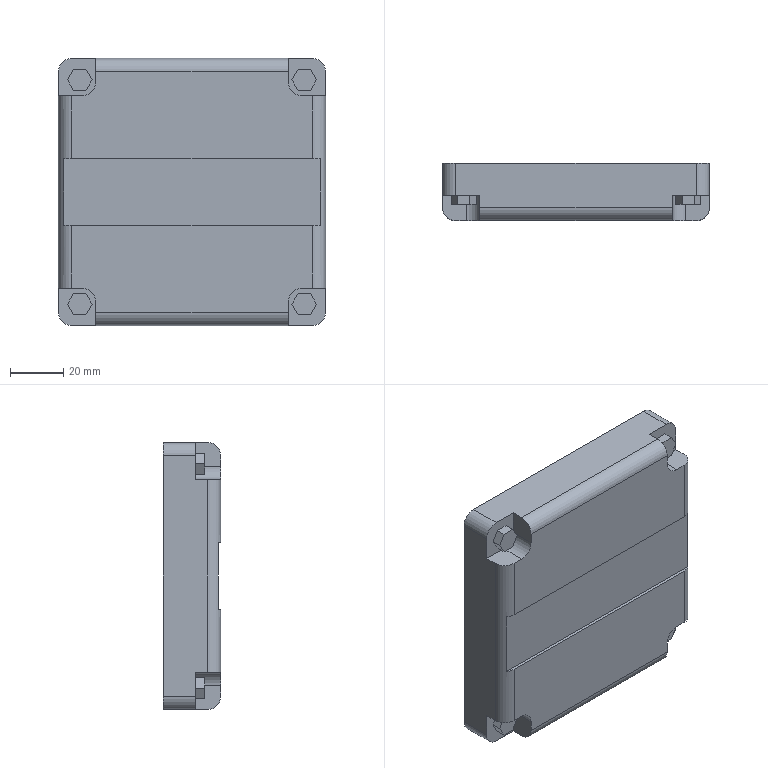Part | STEP file | PRODUCT_NAME_43_default | 1 solid | 62 faces | box 100 x 21.5 x 100 mm | volume 204377 mm3 | plane 50 | cylinder 12 | commonest cylinder face diameters 10 x12